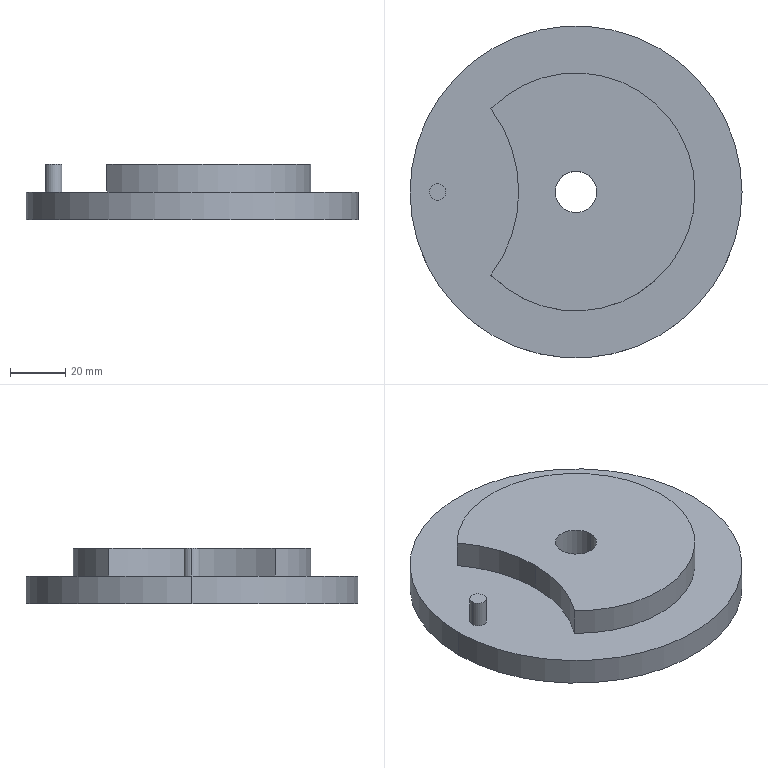Part | STEP file | 1 solid | 14 faces | box 120 x 120 x 20 mm | volume 158754 mm3 | cylinder 10 | plane 4 | commonest cylinder face diameters 6 x2 15 x2 86 x2 100 x2 120 x2
STEP:
#1=CARTESIAN_POINT('',(0.,0.,0.));
#2=DIRECTION('',(0.,0.,1.));
#3=DIRECTION('',(1.,0.,0.));
#4=AXIS2_PLACEMENT_3D('',#1,#2,#3);
#5=CARTESIAN_POINT('',(63.211,0.,10.));
#6=VERTEX_POINT('',#5);
#7=CARTESIAN_POINT('',(63.211,0.,-10.));
#8=VERTEX_POINT('',#7);
#9=CARTESIAN_POINT('',(63.211,0.,-83.));
#10=DIRECTION('',(0.,0.,-1.));
#11=VECTOR('',#10,1.);
#12=LINE('',#9,#11);
#13=CARTESIAN_POINT('',(70.711,0.,-83.));
#14=DIRECTION('',(0.,0.,-1.));
#15=DIRECTION('',(-1.,0.,0.));
#16=AXIS2_PLACEMENT_3D('',#13,#14,#15);
#17=CYLINDRICAL_SURFACE('',#16,7.5);
#18=CARTESIAN_POINT('',(6.283,0.));
#19=DIRECTION('',(0.,1.));
#20=VECTOR('',#19,1.);
#21=LINE('',#18,#20);
#22=(GEOMETRIC_REPRESENTATION_CONTEXT(2)PARAMETRIC_REPRESENTATION_CONTEXT()REPRESENTATION_CONTEXT('',''));
#23=DEFINITIONAL_REPRESENTATION('',(#21),#22);
#24=PCURVE('',#17,#23);
#25=CARTESIAN_POINT('',(70.711,0.,-83.));
#26=DIRECTION('',(0.,0.,-1.));
#27=DIRECTION('',(-1.,0.,0.));
#28=AXIS2_PLACEMENT_3D('',#25,#26,#27);
#29=CYLINDRICAL_SURFACE('',#28,7.5);
#30=CARTESIAN_POINT('',(0.,0.));
#31=DIRECTION('',(0.,1.));
#32=VECTOR('',#31,1.);
#33=LINE('',#30,#32);
#34=(GEOMETRIC_REPRESENTATION_CONTEXT(2)PARAMETRIC_REPRESENTATION_CONTEXT()REPRESENTATION_CONTEXT('',''));
#35=DEFINITIONAL_REPRESENTATION('',(#33),#34);
#36=PCURVE('',#29,#35);
#37=SURFACE_CURVE('',#12,(#24,#36),.PCURVE_S1.);
#38=EDGE_CURVE('',#6,#8,#37,.T.);
#39=ORIENTED_EDGE('',*,*,#38,.T.);
#40=CARTESIAN_POINT('',(78.211,0.,-10.));
#41=VERTEX_POINT('',#40);
#42=CARTESIAN_POINT('',(70.711,0.,-10.));
#43=DIRECTION('',(0.,0.,1.));
#44=DIRECTION('',(-1.,0.,0.));
#45=AXIS2_PLACEMENT_3D('',#42,#43,#44);
#46=CIRCLE('',#45,7.5);
#47=CARTESIAN_POINT('',(6.283,-73.));
#48=DIRECTION('',(-1.,0.));
#49=VECTOR('',#48,1.);
#50=LINE('',#47,#49);
#51=(GEOMETRIC_REPRESENTATION_CONTEXT(2)PARAMETRIC_REPRESENTATION_CONTEXT()REPRESENTATION_CONTEXT('',''));
#52=DEFINITIONAL_REPRESENTATION('',(#50),#51);
#53=PCURVE('',#17,#52);
#54=CARTESIAN_POINT('',(70.711,0.,-10.));
#55=DIRECTION('',(0.,0.,-1.));
#56=DIRECTION('',(-1.,0.,0.));
#57=AXIS2_PLACEMENT_3D('',#54,#55,#56);
#58=PLANE('',#57);
#59=CARTESIAN_POINT('',(7.5,0.));
#60=CARTESIAN_POINT('',(7.5,-12.99));
#61=CARTESIAN_POINT('',(-3.75,-6.495));
#62=CARTESIAN_POINT('',(-15.,0.));
#63=CARTESIAN_POINT('',(-3.75,6.495));
#64=CARTESIAN_POINT('',(7.5,12.99));
#65=CARTESIAN_POINT('',(7.5,0.));
#66=(BOUNDED_CURVE()B_SPLINE_CURVE(2,(#59,#60,#61,#62,#63,#64,#65),.UNSPECIFIED.,.T.,.F.)B_SPLINE_CURVE_WITH_KNOTS((1,2,2,2,2,1),(-2.094,0.,2.094,4.189,6.283,8.378),.UNSPECIFIED.)CURVE()GEOMETRIC_REPRESENTATION_ITEM()RATIONAL_B_SPLINE_CURVE((1.,0.5,1.,0.5,1.,0.5,1.))REPRESENTATION_ITEM(''));
#67=(GEOMETRIC_REPRESENTATION_CONTEXT(2)PARAMETRIC_REPRESENTATION_CONTEXT()REPRESENTATION_CONTEXT('',''));
#68=DEFINITIONAL_REPRESENTATION('',(#66),#67);
#69=PCURVE('',#58,#68);
#70=SURFACE_CURVE('',#46,(#53,#69),.PCURVE_S1.);
#71=EDGE_CURVE('',#8,#41,#70,.T.);
#72=ORIENTED_EDGE('',*,*,#71,.T.);
#73=CARTESIAN_POINT('',(78.211,0.,10.));
#74=VERTEX_POINT('',#73);
#75=CARTESIAN_POINT('',(78.211,0.,-83.));
#76=DIRECTION('',(0.,0.,-1.));
#77=VECTOR('',#76,1.);
#78=LINE('',#75,#77);
#79=CARTESIAN_POINT('',(3.142,0.));
#80=DIRECTION('',(0.,1.));
#81=VECTOR('',#80,1.);
#82=LINE('',#79,#81);
#83=(GEOMETRIC_REPRESENTATION_CONTEXT(2)PARAMETRIC_REPRESENTATION_CONTEXT()REPRESENTATION_CONTEXT('',''));
#84=DEFINITIONAL_REPRESENTATION('',(#82),#83);
#85=PCURVE('',#17,#84);
#86=CARTESIAN_POINT('',(3.142,0.));
#87=DIRECTION('',(0.,1.));
#88=VECTOR('',#87,1.);
#89=LINE('',#86,#88);
#90=(GEOMETRIC_REPRESENTATION_CONTEXT(2)PARAMETRIC_REPRESENTATION_CONTEXT()REPRESENTATION_CONTEXT('',''));
#91=DEFINITIONAL_REPRESENTATION('',(#89),#90);
#92=PCURVE('',#29,#91);
#93=SURFACE_CURVE('',#78,(#85,#92),.PCURVE_S1.);
#94=EDGE_CURVE('',#74,#41,#93,.T.);
#95=ORIENTED_EDGE('',*,*,#94,.F.);
#96=CARTESIAN_POINT('',(70.711,0.,10.));
#97=DIRECTION('',(0.,0.,-1.));
#98=DIRECTION('',(-1.,0.,0.));
#99=AXIS2_PLACEMENT_3D('',#96,#97,#98);
#100=CIRCLE('',#99,7.5);
#101=CARTESIAN_POINT('',(0.,-93.));
#102=DIRECTION('',(1.,0.));
#103=VECTOR('',#102,1.);
#104=LINE('',#101,#103);
#105=(GEOMETRIC_REPRESENTATION_CONTEXT(2)PARAMETRIC_REPRESENTATION_CONTEXT()REPRESENTATION_CONTEXT('',''));
#106=DEFINITIONAL_REPRESENTATION('',(#104),#105);
#107=PCURVE('',#17,#106);
#108=CARTESIAN_POINT('',(0.,0.,10.));
#109=DIRECTION('',(0.,0.,1.));
#110=DIRECTION('',(1.,0.,0.));
#111=AXIS2_PLACEMENT_3D('',#108,#109,#110);
#112=PLANE('',#111);
#113=CARTESIAN_POINT('',(63.211,0.));
#114=CARTESIAN_POINT('',(63.211,12.99));
#115=CARTESIAN_POINT('',(74.461,6.495));
#116=CARTESIAN_POINT('',(85.711,0.));
#117=CARTESIAN_POINT('',(74.461,-6.495));
#118=CARTESIAN_POINT('',(63.211,-12.99));
#119=CARTESIAN_POINT('',(63.211,0.));
#120=(BOUNDED_CURVE()B_SPLINE_CURVE(2,(#113,#114,#115,#116,#117,#118,#119),.UNSPECIFIED.,.T.,.F.)B_SPLINE_CURVE_WITH_KNOTS((1,2,2,2,2,1),(-2.094,0.,2.094,4.189,6.283,8.378),.UNSPECIFIED.)CURVE()GEOMETRIC_REPRESENTATION_ITEM()RATIONAL_B_SPLINE_CURVE((1.,0.5,1.,0.5,1.,0.5,1.))REPRESENTATION_ITEM(''));
#121=(GEOMETRIC_REPRESENTATION_CONTEXT(2)PARAMETRIC_REPRESENTATION_CONTEXT()REPRESENTATION_CONTEXT('',''));
#122=DEFINITIONAL_REPRESENTATION('',(#120),#121);
#123=PCURVE('',#112,#122);
#124=SURFACE_CURVE('',#100,(#107,#123),.PCURVE_S1.);
#125=EDGE_CURVE('',#74,#6,#124,.T.);
#126=ORIENTED_EDGE('',*,*,#125,.T.);
#127=EDGE_LOOP('',(#39,#72,#95,#126));
#128=FACE_BOUND('',#127,.F.);
#129=ADVANCED_FACE('',(#128),#17,.F.);
#130=CARTESIAN_POINT('',(10.711,0.,0.));
#131=VERTEX_POINT('',#130);
#132=CARTESIAN_POINT('',(130.711,0.,0.));
#133=VERTEX_POINT('',#132);
#134=CARTESIAN_POINT('',(70.711,0.,0.));
#135=DIRECTION('',(0.,0.,-1.));
#136=DIRECTION('',(-1.,0.,0.));
#137=AXIS2_PLACEMENT_3D('',#134,#135,#136);
#138=CIRCLE('',#137,60.);
#139=CARTESIAN_POINT('',(70.711,0.,-10.));
#140=DIRECTION('',(0.,0.,-1.));
#141=DIRECTION('',(-1.,0.,0.));
#142=AXIS2_PLACEMENT_3D('',#139,#140,#141);
#143=CYLINDRICAL_SURFACE('',#142,60.);
#144=CARTESIAN_POINT('',(0.,-10.));
#145=DIRECTION('',(1.,0.));
#146=VECTOR('',#145,1.);
#147=LINE('',#144,#146);
#148=(GEOMETRIC_REPRESENTATION_CONTEXT(2)PARAMETRIC_REPRESENTATION_CONTEXT()REPRESENTATION_CONTEXT('',''));
#149=DEFINITIONAL_REPRESENTATION('',(#147),#148);
#150=PCURVE('',#143,#149);
#151=CARTESIAN_POINT('',(70.711,0.,0.));
#152=DIRECTION('',(0.,0.,-1.));
#153=DIRECTION('',(-1.,0.,0.));
#154=AXIS2_PLACEMENT_3D('',#151,#152,#153);
#155=PLANE('',#154);
#156=CARTESIAN_POINT('',(0.,0.));
#157=DIRECTION('',(1.,0.));
#158=AXIS2_PLACEMENT_2D('',#156,#157);
#159=CIRCLE('',#158,60.);
#160=(GEOMETRIC_REPRESENTATION_CONTEXT(2)PARAMETRIC_REPRESENTATION_CONTEXT()REPRESENTATION_CONTEXT('',''));
#161=DEFINITIONAL_REPRESENTATION('',(#159),#160);
#162=PCURVE('',#155,#161);
#163=SURFACE_CURVE('',#138,(#150,#162),.PCURVE_S1.);
#164=EDGE_CURVE('',#131,#133,#163,.T.);
#165=ORIENTED_EDGE('',*,*,#164,.T.);
#166=CARTESIAN_POINT('',(130.711,0.,-10.));
#167=VERTEX_POINT('',#166);
#168=CARTESIAN_POINT('',(130.711,0.,-10.));
#169=DIRECTION('',(0.,0.,-1.));
#170=VECTOR('',#169,1.);
#171=LINE('',#168,#170);
#172=CARTESIAN_POINT('',(3.142,0.));
#173=DIRECTION('',(0.,1.));
#174=VECTOR('',#173,1.);
#175=LINE('',#172,#174);
#176=(GEOMETRIC_REPRESENTATION_CONTEXT(2)PARAMETRIC_REPRESENTATION_CONTEXT()REPRESENTATION_CONTEXT('',''));
#177=DEFINITIONAL_REPRESENTATION('',(#175),#176);
#178=PCURVE('',#143,#177);
#179=CARTESIAN_POINT('',(70.711,0.,-10.));
#180=DIRECTION('',(0.,0.,-1.));
#181=DIRECTION('',(-1.,0.,0.));
#182=AXIS2_PLACEMENT_3D('',#179,#180,#181);
#183=CYLINDRICAL_SURFACE('',#182,60.);
#184=CARTESIAN_POINT('',(3.142,0.));
#185=DIRECTION('',(0.,1.));
#186=VECTOR('',#185,1.);
#187=LINE('',#184,#186);
#188=(GEOMETRIC_REPRESENTATION_CONTEXT(2)PARAMETRIC_REPRESENTATION_CONTEXT()REPRESENTATION_CONTEXT('',''));
#189=DEFINITIONAL_REPRESENTATION('',(#187),#188);
#190=PCURVE('',#183,#189);
#191=SURFACE_CURVE('',#171,(#178,#190),.PCURVE_S1.);
#192=EDGE_CURVE('',#133,#167,#191,.T.);
#193=ORIENTED_EDGE('',*,*,#192,.T.);
#194=CARTESIAN_POINT('',(10.711,0.,-10.));
#195=VERTEX_POINT('',#194);
#196=CARTESIAN_POINT('',(70.711,0.,-10.));
#197=DIRECTION('',(0.,0.,-1.));
#198=DIRECTION('',(-1.,0.,0.));
#199=AXIS2_PLACEMENT_3D('',#196,#197,#198);
#200=CIRCLE('',#199,60.);
#201=CARTESIAN_POINT('',(0.,0.));
#202=DIRECTION('',(1.,0.));
#203=VECTOR('',#202,1.);
#204=LINE('',#201,#203);
#205=(GEOMETRIC_REPRESENTATION_CONTEXT(2)PARAMETRIC_REPRESENTATION_CONTEXT()REPRESENTATION_CONTEXT('',''));
#206=DEFINITIONAL_REPRESENTATION('',(#204),#205);
#207=PCURVE('',#143,#206);
#208=CARTESIAN_POINT('',(0.,0.));
#209=DIRECTION('',(1.,0.));
#210=AXIS2_PLACEMENT_2D('',#208,#209);
#211=CIRCLE('',#210,60.);
#212=(GEOMETRIC_REPRESENTATION_CONTEXT(2)PARAMETRIC_REPRESENTATION_CONTEXT()REPRESENTATION_CONTEXT('',''));
#213=DEFINITIONAL_REPRESENTATION('',(#211),#212);
#214=PCURVE('',#58,#213);
#215=SURFACE_CURVE('',#200,(#207,#214),.PCURVE_S1.);
#216=EDGE_CURVE('',#195,#167,#215,.T.);
#217=ORIENTED_EDGE('',*,*,#216,.F.);
#218=CARTESIAN_POINT('',(10.711,0.,-10.));
#219=DIRECTION('',(0.,0.,-1.));
#220=VECTOR('',#219,1.);
#221=LINE('',#218,#220);
#222=CARTESIAN_POINT('',(0.,0.));
#223=DIRECTION('',(0.,1.));
#224=VECTOR('',#223,1.);
#225=LINE('',#222,#224);
#226=(GEOMETRIC_REPRESENTATION_CONTEXT(2)PARAMETRIC_REPRESENTATION_CONTEXT()REPRESENTATION_CONTEXT('',''));
#227=DEFINITIONAL_REPRESENTATION('',(#225),#226);
#228=PCURVE('',#143,#227);
#229=CARTESIAN_POINT('',(6.283,0.));
#230=DIRECTION('',(0.,1.));
#231=VECTOR('',#230,1.);
#232=LINE('',#229,#231);
#233=(GEOMETRIC_REPRESENTATION_CONTEXT(2)PARAMETRIC_REPRESENTATION_CONTEXT()REPRESENTATION_CONTEXT('',''));
#234=DEFINITIONAL_REPRESENTATION('',(#232),#233);
#235=PCURVE('',#183,#234);
#236=SURFACE_CURVE('',#221,(#228,#235),.PCURVE_S1.);
#237=EDGE_CURVE('',#131,#195,#236,.T.);
#238=ORIENTED_EDGE('',*,*,#237,.F.);
#239=EDGE_LOOP('',(#165,#193,#217,#238));
#240=FACE_BOUND('',#239,.T.);
#241=ADVANCED_FACE('',(#240),#143,.T.);
#242=CARTESIAN_POINT('',(39.959,30.055,0.));
#243=VERTEX_POINT('',#242);
#244=CARTESIAN_POINT('',(39.959,30.055,10.));
#245=VERTEX_POINT('',#244);
#246=CARTESIAN_POINT('',(39.959,30.055,10.));
#247=DIRECTION('',(0.,0.,1.));
#248=VECTOR('',#247,1.);
#249=LINE('',#246,#248);
#250=CARTESIAN_POINT('',(0.,0.,10.));
#251=DIRECTION('',(0.,0.,1.));
#252=DIRECTION('',(1.,0.,0.));
#253=AXIS2_PLACEMENT_3D('',#250,#251,#252);
#254=CYLINDRICAL_SURFACE('',#253,50.);
#255=CARTESIAN_POINT('',(0.6449,0.));
#256=DIRECTION('',(0.,1.));
#257=VECTOR('',#256,1.);
#258=LINE('',#255,#257);
#259=(GEOMETRIC_REPRESENTATION_CONTEXT(2)PARAMETRIC_REPRESENTATION_CONTEXT()REPRESENTATION_CONTEXT('',''));
#260=DEFINITIONAL_REPRESENTATION('',(#258),#259);
#261=PCURVE('',#254,#260);
#262=CARTESIAN_POINT('',(70.711,0.,10.));
#263=DIRECTION('',(0.,0.,1.));
#264=DIRECTION('',(1.,0.,0.));
#265=AXIS2_PLACEMENT_3D('',#262,#263,#264);
#266=CYLINDRICAL_SURFACE('',#265,43.);
#267=CARTESIAN_POINT('',(2.368,0.));
#268=DIRECTION('',(0.,1.));
#269=VECTOR('',#268,1.);
#270=LINE('',#267,#269);
#271=(GEOMETRIC_REPRESENTATION_CONTEXT(2)PARAMETRIC_REPRESENTATION_CONTEXT()REPRESENTATION_CONTEXT('',''));
#272=DEFINITIONAL_REPRESENTATION('',(#270),#271);
#273=PCURVE('',#266,#272);
#274=SURFACE_CURVE('',#249,(#261,#273),.PCURVE_S1.);
#275=EDGE_CURVE('',#243,#245,#274,.T.);
#276=ORIENTED_EDGE('',*,*,#275,.T.);
#277=CARTESIAN_POINT('',(50.,0.,10.));
#278=VERTEX_POINT('',#277);
#279=CARTESIAN_POINT('',(0.,0.,10.));
#280=DIRECTION('',(0.,0.,-1.));
#281=DIRECTION('',(1.,0.,0.));
#282=AXIS2_PLACEMENT_3D('',#279,#280,#281);
#283=CIRCLE('',#282,50.);
#284=CARTESIAN_POINT('',(6.283,0.));
#285=DIRECTION('',(-1.,0.));
#286=VECTOR('',#285,1.);
#287=LINE('',#284,#286);
#288=(GEOMETRIC_REPRESENTATION_CONTEXT(2)PARAMETRIC_REPRESENTATION_CONTEXT()REPRESENTATION_CONTEXT('',''));
#289=DEFINITIONAL_REPRESENTATION('',(#287),#288);
#290=PCURVE('',#254,#289);
#291=CARTESIAN_POINT('',(50.,0.));
#292=CARTESIAN_POINT('',(50.,-86.603));
#293=CARTESIAN_POINT('',(-25.,-43.301));
#294=CARTESIAN_POINT('',(-100.,0.));
#295=CARTESIAN_POINT('',(-25.,43.301));
#296=CARTESIAN_POINT('',(50.,86.603));
#297=CARTESIAN_POINT('',(50.,0.));
#298=(BOUNDED_CURVE()B_SPLINE_CURVE(2,(#291,#292,#293,#294,#295,#296,#297),.UNSPECIFIED.,.T.,.F.)B_SPLINE_CURVE_WITH_KNOTS((1,2,2,2,2,1),(-2.094,0.,2.094,4.189,6.283,8.378),.UNSPECIFIED.)CURVE()GEOMETRIC_REPRESENTATION_ITEM()RATIONAL_B_SPLINE_CURVE((1.,0.5,1.,0.5,1.,0.5,1.))REPRESENTATION_ITEM(''));
#299=(GEOMETRIC_REPRESENTATION_CONTEXT(2)PARAMETRIC_REPRESENTATION_CONTEXT()REPRESENTATION_CONTEXT('',''));
#300=DEFINITIONAL_REPRESENTATION('',(#298),#299);
#301=PCURVE('',#112,#300);
#302=SURFACE_CURVE('',#283,(#290,#301),.PCURVE_S1.);
#303=EDGE_CURVE('',#245,#278,#302,.T.);
#304=ORIENTED_EDGE('',*,*,#303,.T.);
#305=CARTESIAN_POINT('',(50.,0.,0.));
#306=VERTEX_POINT('',#305);
#307=CARTESIAN_POINT('',(50.,0.,10.));
#308=DIRECTION('',(0.,0.,1.));
#309=VECTOR('',#308,1.);
#310=LINE('',#307,#309);
#311=CARTESIAN_POINT('',(0.,0.));
#312=DIRECTION('',(0.,1.));
#313=VECTOR('',#312,1.);
#314=LINE('',#311,#313);
#315=(GEOMETRIC_REPRESENTATION_CONTEXT(2)PARAMETRIC_REPRESENTATION_CONTEXT()REPRESENTATION_CONTEXT('',''));
#316=DEFINITIONAL_REPRESENTATION('',(#314),#315);
#317=PCURVE('',#254,#316);
#318=CARTESIAN_POINT('',(0.,0.,10.));
#319=DIRECTION('',(0.,0.,1.));
#320=DIRECTION('',(1.,0.,0.));
#321=AXIS2_PLACEMENT_3D('',#318,#319,#320);
#322=CYLINDRICAL_SURFACE('',#321,50.);
#323=CARTESIAN_POINT('',(6.283,0.));
#324=DIRECTION('',(0.,1.));
#325=VECTOR('',#324,1.);
#326=LINE('',#323,#325);
#327=(GEOMETRIC_REPRESENTATION_CONTEXT(2)PARAMETRIC_REPRESENTATION_CONTEXT()REPRESENTATION_CONTEXT('',''));
#328=DEFINITIONAL_REPRESENTATION('',(#326),#327);
#329=PCURVE('',#322,#328);
#330=SURFACE_CURVE('',#310,(#317,#329),.PCURVE_S1.);
#331=EDGE_CURVE('',#306,#278,#330,.T.);
#332=ORIENTED_EDGE('',*,*,#331,.F.);
#333=CARTESIAN_POINT('',(0.,0.,0.));
#334=DIRECTION('',(0.,0.,-1.));
#335=DIRECTION('',(1.,0.,0.));
#336=AXIS2_PLACEMENT_3D('',#333,#334,#335);
#337=CIRCLE('',#336,50.);
#338=CARTESIAN_POINT('',(6.283,-10.));
#339=DIRECTION('',(-1.,0.));
#340=VECTOR('',#339,1.);
#341=LINE('',#338,#340);
#342=(GEOMETRIC_REPRESENTATION_CONTEXT(2)PARAMETRIC_REPRESENTATION_CONTEXT()REPRESENTATION_CONTEXT('',''));
#343=DEFINITIONAL_REPRESENTATION('',(#341),#342);
#344=PCURVE('',#254,#343);
#345=CARTESIAN_POINT('',(70.711,0.));
#346=DIRECTION('',(-1.,0.));
#347=AXIS2_PLACEMENT_2D('',#345,#346);
#348=CIRCLE('',#347,50.);
#349=(GEOMETRIC_REPRESENTATION_CONTEXT(2)PARAMETRIC_REPRESENTATION_CONTEXT()REPRESENTATION_CONTEXT('',''));
#350=DEFINITIONAL_REPRESENTATION('',(#348),#349);
#351=PCURVE('',#155,#350);
#352=SURFACE_CURVE('',#337,(#344,#351),.PCURVE_S1.);
#353=EDGE_CURVE('',#243,#306,#352,.T.);
#354=ORIENTED_EDGE('',*,*,#353,.F.);
#355=EDGE_LOOP('',(#276,#304,#332,#354));
#356=FACE_BOUND('',#355,.F.);
#357=ADVANCED_FACE('',(#356),#254,.F.);
#358=CARTESIAN_POINT('',(39.959,-30.055,0.));
#359=VERTEX_POINT('',#358);
#360=CARTESIAN_POINT('',(113.711,0.,0.));
#361=VERTEX_POINT('',#360);
#362=CARTESIAN_POINT('',(70.711,0.,0.));
#363=DIRECTION('',(0.,0.,1.));
#364=DIRECTION('',(1.,0.,0.));
#365=AXIS2_PLACEMENT_3D('',#362,#363,#364);
#366=CIRCLE('',#365,43.);
#367=CARTESIAN_POINT('',(70.711,0.,10.));
#368=DIRECTION('',(0.,0.,1.));
#369=DIRECTION('',(1.,0.,0.));
#370=AXIS2_PLACEMENT_3D('',#367,#368,#369);
#371=CYLINDRICAL_SURFACE('',#370,43.);
#372=CARTESIAN_POINT('',(0.,-10.));
#373=DIRECTION('',(1.,0.));
#374=VECTOR('',#373,1.);
#375=LINE('',#372,#374);
#376=(GEOMETRIC_REPRESENTATION_CONTEXT(2)PARAMETRIC_REPRESENTATION_CONTEXT()REPRESENTATION_CONTEXT('',''));
#377=DEFINITIONAL_REPRESENTATION('',(#375),#376);
#378=PCURVE('',#371,#377);
#379=CARTESIAN_POINT('',(-43.,0.));
#380=CARTESIAN_POINT('',(-43.,74.478));
#381=CARTESIAN_POINT('',(21.5,37.239));
#382=CARTESIAN_POINT('',(86.,0.));
#383=CARTESIAN_POINT('',(21.5,-37.239));
#384=CARTESIAN_POINT('',(-43.,-74.478));
#385=CARTESIAN_POINT('',(-43.,0.));
#386=(BOUNDED_CURVE()B_SPLINE_CURVE(2,(#379,#380,#381,#382,#383,#384,#385),.UNSPECIFIED.,.T.,.F.)B_SPLINE_CURVE_WITH_KNOTS((1,2,2,2,2,1),(-2.094,0.,2.094,4.189,6.283,8.378),.UNSPECIFIED.)CURVE()GEOMETRIC_REPRESENTATION_ITEM()RATIONAL_B_SPLINE_CURVE((1.,0.5,1.,0.5,1.,0.5,1.))REPRESENTATION_ITEM(''));
#387=(GEOMETRIC_REPRESENTATION_CONTEXT(2)PARAMETRIC_REPRESENTATION_CONTEXT()REPRESENTATION_CONTEXT('',''));
#388=DEFINITIONAL_REPRESENTATION('',(#386),#387);
#389=PCURVE('',#155,#388);
#390=SURFACE_CURVE('',#366,(#378,#389),.PCURVE_S1.);
#391=EDGE_CURVE('',#359,#361,#390,.T.);
#392=ORIENTED_EDGE('',*,*,#391,.T.);
#393=CARTESIAN_POINT('',(113.711,0.,10.));
#394=VERTEX_POINT('',#393);
#395=CARTESIAN_POINT('',(113.711,0.,10.));
#396=DIRECTION('',(0.,0.,1.));
#397=VECTOR('',#396,1.);
#398=LINE('',#395,#397);
#399=CARTESIAN_POINT('',(6.283,0.));
#400=DIRECTION('',(0.,1.));
#401=VECTOR('',#400,1.);
#402=LINE('',#399,#401);
#403=(GEOMETRIC_REPRESENTATION_CONTEXT(2)PARAMETRIC_REPRESENTATION_CONTEXT()REPRESENTATION_CONTEXT('',''));
#404=DEFINITIONAL_REPRESENTATION('',(#402),#403);
#405=PCURVE('',#371,#404);
#406=CARTESIAN_POINT('',(0.,0.));
#407=DIRECTION('',(0.,1.));
#408=VECTOR('',#407,1.);
#409=LINE('',#406,#408);
#410=(GEOMETRIC_REPRESENTATION_CONTEXT(2)PARAMETRIC_REPRESENTATION_CONTEXT()REPRESENTATION_CONTEXT('',''));
#411=DEFINITIONAL_REPRESENTATION('',(#409),#410);
#412=PCURVE('',#266,#411);
#413=SURFACE_CURVE('',#398,(#405,#412),.PCURVE_S1.);
#414=EDGE_CURVE('',#361,#394,#413,.T.);
#415=ORIENTED_EDGE('',*,*,#414,.T.);
#416=CARTESIAN_POINT('',(39.959,-30.055,10.));
#417=VERTEX_POINT('',#416);
#418=CARTESIAN_POINT('',(70.711,0.,10.));
#419=DIRECTION('',(0.,0.,1.));
#420=DIRECTION('',(1.,0.,0.));
#421=AXIS2_PLACEMENT_3D('',#418,#419,#420);
#422=CIRCLE('',#421,43.);
#423=CARTESIAN_POINT('',(0.,0.));
#424=DIRECTION('',(1.,0.));
#425=VECTOR('',#424,1.);
#426=LINE('',#423,#425);
#427=(GEOMETRIC_REPRESENTATION_CONTEXT(2)PARAMETRIC_REPRESENTATION_CONTEXT()REPRESENTATION_CONTEXT('',''));
#428=DEFINITIONAL_REPRESENTATION('',(#426),#427);
#429=PCURVE('',#371,#428);
#430=CARTESIAN_POINT('',(70.711,0.));
#431=DIRECTION('',(1.,0.));
#432=AXIS2_PLACEMENT_2D('',#430,#431);
#433=CIRCLE('',#432,43.);
#434=(GEOMETRIC_REPRESENTATION_CONTEXT(2)PARAMETRIC_REPRESENTATION_CONTEXT()REPRESENTATION_CONTEXT('',''));
#435=DEFINITIONAL_REPRESENTATION('',(#433),#434);
#436=PCURVE('',#112,#435);
#437=SURFACE_CURVE('',#422,(#429,#436),.PCURVE_S1.);
#438=EDGE_CURVE('',#417,#394,#437,.T.);
#439=ORIENTED_EDGE('',*,*,#438,.F.);
#440=CARTESIAN_POINT('',(39.959,-30.055,10.));
#441=DIRECTION('',(0.,0.,-1.));
#442=VECTOR('',#441,1.);
#443=LINE('',#440,#442);
#444=CARTESIAN_POINT('',(3.916,0.));
#445=DIRECTION('',(0.,-1.));
#446=VECTOR('',#445,1.);
#447=LINE('',#444,#446);
#448=(GEOMETRIC_REPRESENTATION_CONTEXT(2)PARAMETRIC_REPRESENTATION_CONTEXT()REPRESENTATION_CONTEXT('',''));
#449=DEFINITIONAL_REPRESENTATION('',(#447),#448);
#450=PCURVE('',#371,#449);
#451=CARTESIAN_POINT('',(5.638,0.));
#452=DIRECTION('',(0.,-1.));
#453=VECTOR('',#452,1.);
#454=LINE('',#451,#453);
#455=(GEOMETRIC_REPRESENTATION_CONTEXT(2)PARAMETRIC_REPRESENTATION_CONTEXT()REPRESENTATION_CONTEXT('',''));
#456=DEFINITIONAL_REPRESENTATION('',(#454),#455);
#457=PCURVE('',#322,#456);
#458=SURFACE_CURVE('',#443,(#450,#457),.PCURVE_S1.);
#459=EDGE_CURVE('',#417,#359,#458,.T.);
#460=ORIENTED_EDGE('',*,*,#459,.T.);
#461=EDGE_LOOP('',(#392,#415,#439,#460));
#462=FACE_BOUND('',#461,.T.);
#463=ADVANCED_FACE('',(#462),#371,.T.);
#464=CARTESIAN_POINT('',(23.711,0.,0.));
#465=VERTEX_POINT('',#464);
#466=CARTESIAN_POINT('',(17.711,0.,0.));
#467=VERTEX_POINT('',#466);
#468=CARTESIAN_POINT('',(20.711,0.,0.));
#469=DIRECTION('',(0.,0.,1.));
#470=DIRECTION('',(1.,0.,0.));
#471=AXIS2_PLACEMENT_3D('',#468,#469,#470);
#472=CIRCLE('',#471,3.);
#473=CARTESIAN_POINT('',(20.711,0.,10.));
#474=DIRECTION('',(0.,0.,1.));
#475=DIRECTION('',(1.,0.,0.));
#476=AXIS2_PLACEMENT_3D('',#473,#474,#475);
#477=CYLINDRICAL_SURFACE('',#476,3.);
#478=CARTESIAN_POINT('',(0.,-10.));
#479=DIRECTION('',(1.,0.));
#480=VECTOR('',#479,1.);
#481=LINE('',#478,#480);
#482=(GEOMETRIC_REPRESENTATION_CONTEXT(2)PARAMETRIC_REPRESENTATION_CONTEXT()REPRESENTATION_CONTEXT('',''));
#483=DEFINITIONAL_REPRESENTATION('',(#481),#482);
#484=PCURVE('',#477,#483);
#485=CARTESIAN_POINT('',(47.,0.));
#486=CARTESIAN_POINT('',(47.,5.196));
#487=CARTESIAN_POINT('',(51.5,2.598));
#488=CARTESIAN_POINT('',(56.,0.));
#489=CARTESIAN_POINT('',(51.5,-2.598));
#490=CARTESIAN_POINT('',(47.,-5.196));
#491=CARTESIAN_POINT('',(47.,0.));
#492=(BOUNDED_CURVE()B_SPLINE_CURVE(2,(#485,#486,#487,#488,#489,#490,#491),.UNSPECIFIED.,.T.,.F.)B_SPLINE_CURVE_WITH_KNOTS((1,2,2,2,2,1),(-2.094,0.,2.094,4.189,6.283,8.378),.UNSPECIFIED.)CURVE()GEOMETRIC_REPRESENTATION_ITEM()RATIONAL_B_SPLINE_CURVE((1.,0.5,1.,0.5,1.,0.5,1.))REPRESENTATION_ITEM(''));
#493=(GEOMETRIC_REPRESENTATION_CONTEXT(2)PARAMETRIC_REPRESENTATION_CONTEXT()REPRESENTATION_CONTEXT('',''));
#494=DEFINITIONAL_REPRESENTATION('',(#492),#493);
#495=PCURVE('',#155,#494);
#496=SURFACE_CURVE('',#472,(#484,#495),.PCURVE_S1.);
#497=EDGE_CURVE('',#465,#467,#496,.T.);
#498=ORIENTED_EDGE('',*,*,#497,.T.);
#499=CARTESIAN_POINT('',(17.711,0.,10.));
#500=VERTEX_POINT('',#499);
#501=CARTESIAN_POINT('',(17.711,0.,10.));
#502=DIRECTION('',(0.,0.,1.));
#503=VECTOR('',#502,1.);
#504=LINE('',#501,#503);
#505=CARTESIAN_POINT('',(3.142,0.));
#506=DIRECTION('',(0.,1.));
#507=VECTOR('',#506,1.);
#508=LINE('',#505,#507);
#509=(GEOMETRIC_REPRESENTATION_CONTEXT(2)PARAMETRIC_REPRESENTATION_CONTEXT()REPRESENTATION_CONTEXT('',''));
#510=DEFINITIONAL_REPRESENTATION('',(#508),#509);
#511=PCURVE('',#477,#510);
#512=CARTESIAN_POINT('',(20.711,0.,10.));
#513=DIRECTION('',(0.,0.,1.));
#514=DIRECTION('',(1.,0.,0.));
#515=AXIS2_PLACEMENT_3D('',#512,#513,#514);
#516=CYLINDRICAL_SURFACE('',#515,3.);
#517=CARTESIAN_POINT('',(3.142,0.));
#518=DIRECTION('',(0.,1.));
#519=VECTOR('',#518,1.);
#520=LINE('',#517,#519);
#521=(GEOMETRIC_REPRESENTATION_CONTEXT(2)PARAMETRIC_REPRESENTATION_CONTEXT()REPRESENTATION_CONTEXT('',''));
#522=DEFINITIONAL_REPRESENTATION('',(#520),#521);
#523=PCURVE('',#516,#522);
#524=SURFACE_CURVE('',#504,(#511,#523),.PCURVE_S1.);
#525=EDGE_CURVE('',#467,#500,#524,.T.);
#526=ORIENTED_EDGE('',*,*,#525,.T.);
#527=CARTESIAN_POINT('',(23.711,0.,10.));
#528=VERTEX_POINT('',#527);
#529=CARTESIAN_POINT('',(20.711,0.,10.));
#530=DIRECTION('',(0.,0.,-1.));
#531=DIRECTION('',(1.,0.,0.));
#532=AXIS2_PLACEMENT_3D('',#529,#530,#531);
#533=CIRCLE('',#532,3.);
#534=CARTESIAN_POINT('',(6.283,0.));
#535=DIRECTION('',(-1.,0.));
#536=VECTOR('',#535,1.);
#537=LINE('',#534,#536);
#538=(GEOMETRIC_REPRESENTATION_CONTEXT(2)PARAMETRIC_REPRESENTATION_CONTEXT()REPRESENTATION_CONTEXT('',''));
#539=DEFINITIONAL_REPRESENTATION('',(#537),#538);
#540=PCURVE('',#477,#539);
#541=CARTESIAN_POINT('',(20.711,0.,10.));
#542=DIRECTION('',(0.,0.,1.));
#543=DIRECTION('',(1.,0.,0.));
#544=AXIS2_PLACEMENT_3D('',#541,#542,#543);
#545=PLANE('',#544);
#546=CARTESIAN_POINT('',(3.,0.));
#547=CARTESIAN_POINT('',(3.,-5.196));
#548=CARTESIAN_POINT('',(-1.5,-2.598));
#549=CARTESIAN_POINT('',(-6.,0.));
#550=CARTESIAN_POINT('',(-1.5,2.598));
#551=CARTESIAN_POINT('',(3.,5.196));
#552=CARTESIAN_POINT('',(3.,0.));
#553=(BOUNDED_CURVE()B_SPLINE_CURVE(2,(#546,#547,#548,#549,#550,#551,#552),.UNSPECIFIED.,.T.,.F.)B_SPLINE_CURVE_WITH_KNOTS((1,2,2,2,2,1),(-2.094,0.,2.094,4.189,6.283,8.378),.UNSPECIFIED.)CURVE()GEOMETRIC_REPRESENTATION_ITEM()RATIONAL_B_SPLINE_CURVE((1.,0.5,1.,0.5,1.,0.5,1.))REPRESENTATION_ITEM(''));
#554=(GEOMETRIC_REPRESENTATION_CONTEXT(2)PARAMETRIC_REPRESENTATION_CONTEXT()REPRESENTATION_CONTEXT('',''));
#555=DEFINITIONAL_REPRESENTATION('',(#553),#554);
#556=PCURVE('',#545,#555);
#557=SURFACE_CURVE('',#533,(#540,#556),.PCURVE_S1.);
#558=EDGE_CURVE('',#500,#528,#557,.T.);
#559=ORIENTED_EDGE('',*,*,#558,.T.);
#560=CARTESIAN_POINT('',(23.711,0.,10.));
#561=DIRECTION('',(0.,0.,1.));
#562=VECTOR('',#561,1.);
#563=LINE('',#560,#562);
#564=CARTESIAN_POINT('',(0.,0.));
#565=DIRECTION('',(0.,1.));
#566=VECTOR('',#565,1.);
#567=LINE('',#564,#566);
#568=(GEOMETRIC_REPRESENTATION_CONTEXT(2)PARAMETRIC_REPRESENTATION_CONTEXT()REPRESENTATION_CONTEXT('',''));
#569=DEFINITIONAL_REPRESENTATION('',(#567),#568);
#570=PCURVE('',#477,#569);
#571=CARTESIAN_POINT('',(6.283,0.));
#572=DIRECTION('',(0.,1.));
#573=VECTOR('',#572,1.);
#574=LINE('',#571,#573);
#575=(GEOMETRIC_REPRESENTATION_CONTEXT(2)PARAMETRIC_REPRESENTATION_CONTEXT()REPRESENTATION_CONTEXT('',''));
#576=DEFINITIONAL_REPRESENTATION('',(#574),#575);
#577=PCURVE('',#516,#576);
#578=SURFACE_CURVE('',#563,(#570,#577),.PCURVE_S1.);
#579=EDGE_CURVE('',#465,#528,#578,.T.);
#580=ORIENTED_EDGE('',*,*,#579,.F.);
#581=EDGE_LOOP('',(#498,#526,#559,#580));
#582=FACE_BOUND('',#581,.T.);
#583=ADVANCED_FACE('',(#582),#477,.T.);
#584=ORIENTED_EDGE('',*,*,#71,.T.);
#585=CARTESIAN_POINT('',(70.711,0.,-10.));
#586=DIRECTION('',(0.,0.,1.));
#587=DIRECTION('',(-1.,0.,0.));
#588=AXIS2_PLACEMENT_3D('',#585,#586,#587);
#589=CIRCLE('',#588,7.5);
#590=CARTESIAN_POINT('',(7.5,0.));
#591=CARTESIAN_POINT('',(7.5,-12.99));
#592=CARTESIAN_POINT('',(-3.75,-6.495));
#593=CARTESIAN_POINT('',(-15.,0.));
#594=CARTESIAN_POINT('',(-3.75,6.495));
#595=CARTESIAN_POINT('',(7.5,12.99));
#596=CARTESIAN_POINT('',(7.5,0.));
#597=(BOUNDED_CURVE()B_SPLINE_CURVE(2,(#590,#591,#592,#593,#594,#595,#596),.UNSPECIFIED.,.T.,.F.)B_SPLINE_CURVE_WITH_KNOTS((1,2,2,2,2,1),(-2.094,0.,2.094,4.189,6.283,8.378),.UNSPECIFIED.)CURVE()GEOMETRIC_REPRESENTATION_ITEM()RATIONAL_B_SPLINE_CURVE((1.,0.5,1.,0.5,1.,0.5,1.))REPRESENTATION_ITEM(''));
#598=(GEOMETRIC_REPRESENTATION_CONTEXT(2)PARAMETRIC_REPRESENTATION_CONTEXT()REPRESENTATION_CONTEXT('',''));
#599=DEFINITIONAL_REPRESENTATION('',(#597),#598);
#600=PCURVE('',#58,#599);
#601=CARTESIAN_POINT('',(6.283,-73.));
#602=DIRECTION('',(-1.,0.));
#603=VECTOR('',#602,1.);
#604=LINE('',#601,#603);
#605=(GEOMETRIC_REPRESENTATION_CONTEXT(2)PARAMETRIC_REPRESENTATION_CONTEXT()REPRESENTATION_CONTEXT('',''));
#606=DEFINITIONAL_REPRESENTATION('',(#604),#605);
#607=PCURVE('',#29,#606);
#608=SURFACE_CURVE('',#589,(#600,#607),.PCURVE_S1.);
#609=EDGE_CURVE('',#41,#8,#608,.T.);
#610=ORIENTED_EDGE('',*,*,#609,.T.);
#611=EDGE_LOOP('',(#584,#610));
#612=FACE_BOUND('',#611,.T.);
#613=ORIENTED_EDGE('',*,*,#216,.T.);
#614=CARTESIAN_POINT('',(70.711,0.,-10.));
#615=DIRECTION('',(0.,0.,-1.));
#616=DIRECTION('',(-1.,0.,0.));
#617=AXIS2_PLACEMENT_3D('',#614,#615,#616);
#618=CIRCLE('',#617,60.);
#619=CARTESIAN_POINT('',(0.,0.));
#620=DIRECTION('',(1.,0.));
#621=AXIS2_PLACEMENT_2D('',#619,#620);
#622=CIRCLE('',#621,60.);
#623=(GEOMETRIC_REPRESENTATION_CONTEXT(2)PARAMETRIC_REPRESENTATION_CONTEXT()REPRESENTATION_CONTEXT('',''));
#624=DEFINITIONAL_REPRESENTATION('',(#622),#623);
#625=PCURVE('',#58,#624);
#626=CARTESIAN_POINT('',(0.,0.));
#627=DIRECTION('',(1.,0.));
#628=VECTOR('',#627,1.);
#629=LINE('',#626,#628);
#630=(GEOMETRIC_REPRESENTATION_CONTEXT(2)PARAMETRIC_REPRESENTATION_CONTEXT()REPRESENTATION_CONTEXT('',''));
#631=DEFINITIONAL_REPRESENTATION('',(#629),#630);
#632=PCURVE('',#183,#631);
#633=SURFACE_CURVE('',#618,(#625,#632),.PCURVE_S1.);
#634=EDGE_CURVE('',#167,#195,#633,.T.);
#635=ORIENTED_EDGE('',*,*,#634,.T.);
#636=EDGE_LOOP('',(#613,#635));
#637=FACE_BOUND('',#636,.T.);
#638=ADVANCED_FACE('',(#612,#637),#58,.T.);
#639=ORIENTED_EDGE('',*,*,#609,.T.);
#640=ORIENTED_EDGE('',*,*,#38,.F.);
#641=CARTESIAN_POINT('',(70.711,0.,10.));
#642=DIRECTION('',(0.,0.,-1.));
#643=DIRECTION('',(-1.,0.,0.));
#644=AXIS2_PLACEMENT_3D('',#641,#642,#643);
#645=CIRCLE('',#644,7.5);
#646=CARTESIAN_POINT('',(0.,-93.));
#647=DIRECTION('',(1.,0.));
#648=VECTOR('',#647,1.);
#649=LINE('',#646,#648);
#650=(GEOMETRIC_REPRESENTATION_CONTEXT(2)PARAMETRIC_REPRESENTATION_CONTEXT()REPRESENTATION_CONTEXT('',''));
#651=DEFINITIONAL_REPRESENTATION('',(#649),#650);
#652=PCURVE('',#29,#651);
#653=CARTESIAN_POINT('',(63.211,0.));
#654=CARTESIAN_POINT('',(63.211,12.99));
#655=CARTESIAN_POINT('',(74.461,6.495));
#656=CARTESIAN_POINT('',(85.711,0.));
#657=CARTESIAN_POINT('',(74.461,-6.495));
#658=CARTESIAN_POINT('',(63.211,-12.99));
#659=CARTESIAN_POINT('',(63.211,0.));
#660=(BOUNDED_CURVE()B_SPLINE_CURVE(2,(#653,#654,#655,#656,#657,#658,#659),.UNSPECIFIED.,.T.,.F.)B_SPLINE_CURVE_WITH_KNOTS((1,2,2,2,2,1),(-2.094,0.,2.094,4.189,6.283,8.378),.UNSPECIFIED.)CURVE()GEOMETRIC_REPRESENTATION_ITEM()RATIONAL_B_SPLINE_CURVE((1.,0.5,1.,0.5,1.,0.5,1.))REPRESENTATION_ITEM(''));
#661=(GEOMETRIC_REPRESENTATION_CONTEXT(2)PARAMETRIC_REPRESENTATION_CONTEXT()REPRESENTATION_CONTEXT('',''));
#662=DEFINITIONAL_REPRESENTATION('',(#660),#661);
#663=PCURVE('',#112,#662);
#664=SURFACE_CURVE('',#645,(#652,#663),.PCURVE_S1.);
#665=EDGE_CURVE('',#6,#74,#664,.T.);
#666=ORIENTED_EDGE('',*,*,#665,.T.);
#667=ORIENTED_EDGE('',*,*,#94,.T.);
#668=EDGE_LOOP('',(#639,#640,#666,#667));
#669=FACE_BOUND('',#668,.F.);
#670=ADVANCED_FACE('',(#669),#29,.F.);
#671=ORIENTED_EDGE('',*,*,#192,.F.);
#672=CARTESIAN_POINT('',(70.711,0.,0.));
#673=DIRECTION('',(0.,0.,-1.));
#674=DIRECTION('',(-1.,0.,0.));
#675=AXIS2_PLACEMENT_3D('',#672,#673,#674);
#676=CIRCLE('',#675,60.);
#677=CARTESIAN_POINT('',(0.,-10.));
#678=DIRECTION('',(1.,0.));
#679=VECTOR('',#678,1.);
#680=LINE('',#677,#679);
#681=(GEOMETRIC_REPRESENTATION_CONTEXT(2)PARAMETRIC_REPRESENTATION_CONTEXT()REPRESENTATION_CONTEXT('',''));
#682=DEFINITIONAL_REPRESENTATION('',(#680),#681);
#683=PCURVE('',#183,#682);
#684=CARTESIAN_POINT('',(0.,0.));
#685=DIRECTION('',(1.,0.));
#686=AXIS2_PLACEMENT_2D('',#684,#685);
#687=CIRCLE('',#686,60.);
#688=(GEOMETRIC_REPRESENTATION_CONTEXT(2)PARAMETRIC_REPRESENTATION_CONTEXT()REPRESENTATION_CONTEXT('',''));
#689=DEFINITIONAL_REPRESENTATION('',(#687),#688);
#690=PCURVE('',#155,#689);
#691=SURFACE_CURVE('',#676,(#683,#690),.PCURVE_S1.);
#692=EDGE_CURVE('',#133,#131,#691,.T.);
#693=ORIENTED_EDGE('',*,*,#692,.T.);
#694=ORIENTED_EDGE('',*,*,#237,.T.);
#695=ORIENTED_EDGE('',*,*,#634,.F.);
#696=EDGE_LOOP('',(#671,#693,#694,#695));
#697=FACE_BOUND('',#696,.T.);
#698=ADVANCED_FACE('',(#697),#183,.T.);
#699=ORIENTED_EDGE('',*,*,#665,.T.);
#700=ORIENTED_EDGE('',*,*,#125,.T.);
#701=EDGE_LOOP('',(#699,#700));
#702=FACE_BOUND('',#701,.T.);
#703=ORIENTED_EDGE('',*,*,#438,.T.);
#704=CARTESIAN_POINT('',(70.711,0.,10.));
#705=DIRECTION('',(0.,0.,1.));
#706=DIRECTION('',(1.,0.,0.));
#707=AXIS2_PLACEMENT_3D('',#704,#705,#706);
#708=CIRCLE('',#707,43.);
#709=CARTESIAN_POINT('',(70.711,0.));
#710=DIRECTION('',(1.,0.));
#711=AXIS2_PLACEMENT_2D('',#709,#710);
#712=CIRCLE('',#711,43.);
#713=(GEOMETRIC_REPRESENTATION_CONTEXT(2)PARAMETRIC_REPRESENTATION_CONTEXT()REPRESENTATION_CONTEXT('',''));
#714=DEFINITIONAL_REPRESENTATION('',(#712),#713);
#715=PCURVE('',#112,#714);
#716=CARTESIAN_POINT('',(0.,0.));
#717=DIRECTION('',(1.,0.));
#718=VECTOR('',#717,1.);
#719=LINE('',#716,#718);
#720=(GEOMETRIC_REPRESENTATION_CONTEXT(2)PARAMETRIC_REPRESENTATION_CONTEXT()REPRESENTATION_CONTEXT('',''));
#721=DEFINITIONAL_REPRESENTATION('',(#719),#720);
#722=PCURVE('',#266,#721);
#723=SURFACE_CURVE('',#708,(#715,#722),.PCURVE_S1.);
#724=EDGE_CURVE('',#394,#245,#723,.T.);
#725=ORIENTED_EDGE('',*,*,#724,.T.);
#726=ORIENTED_EDGE('',*,*,#303,.T.);
#727=CARTESIAN_POINT('',(0.,0.,10.));
#728=DIRECTION('',(0.,0.,-1.));
#729=DIRECTION('',(1.,0.,0.));
#730=AXIS2_PLACEMENT_3D('',#727,#728,#729);
#731=CIRCLE('',#730,50.);
#732=CARTESIAN_POINT('',(50.,0.));
#733=CARTESIAN_POINT('',(50.,-86.603));
#734=CARTESIAN_POINT('',(-25.,-43.301));
#735=CARTESIAN_POINT('',(-100.,0.));
#736=CARTESIAN_POINT('',(-25.,43.301));
#737=CARTESIAN_POINT('',(50.,86.603));
#738=CARTESIAN_POINT('',(50.,0.));
#739=(BOUNDED_CURVE()B_SPLINE_CURVE(2,(#732,#733,#734,#735,#736,#737,#738),.UNSPECIFIED.,.T.,.F.)B_SPLINE_CURVE_WITH_KNOTS((1,2,2,2,2,1),(-2.094,0.,2.094,4.189,6.283,8.378),.UNSPECIFIED.)CURVE()GEOMETRIC_REPRESENTATION_ITEM()RATIONAL_B_SPLINE_CURVE((1.,0.5,1.,0.5,1.,0.5,1.))REPRESENTATION_ITEM(''));
#740=(GEOMETRIC_REPRESENTATION_CONTEXT(2)PARAMETRIC_REPRESENTATION_CONTEXT()REPRESENTATION_CONTEXT('',''));
#741=DEFINITIONAL_REPRESENTATION('',(#739),#740);
#742=PCURVE('',#112,#741);
#743=CARTESIAN_POINT('',(6.283,0.));
#744=DIRECTION('',(-1.,0.));
#745=VECTOR('',#744,1.);
#746=LINE('',#743,#745);
#747=(GEOMETRIC_REPRESENTATION_CONTEXT(2)PARAMETRIC_REPRESENTATION_CONTEXT()REPRESENTATION_CONTEXT('',''));
#748=DEFINITIONAL_REPRESENTATION('',(#746),#747);
#749=PCURVE('',#322,#748);
#750=SURFACE_CURVE('',#731,(#742,#749),.PCURVE_S1.);
#751=EDGE_CURVE('',#278,#417,#750,.T.);
#752=ORIENTED_EDGE('',*,*,#751,.T.);
#753=EDGE_LOOP('',(#703,#725,#726,#752));
#754=FACE_BOUND('',#753,.T.);
#755=ADVANCED_FACE('',(#702,#754),#112,.T.);
#756=ORIENTED_EDGE('',*,*,#353,.F.);
#757=CARTESIAN_POINT('',(70.711,0.,0.));
#758=DIRECTION('',(0.,0.,1.));
#759=DIRECTION('',(1.,0.,0.));
#760=AXIS2_PLACEMENT_3D('',#757,#758,#759);
#761=CIRCLE('',#760,43.);
#762=CARTESIAN_POINT('',(-43.,0.));
#763=CARTESIAN_POINT('',(-43.,74.478));
#764=CARTESIAN_POINT('',(21.5,37.239));
#765=CARTESIAN_POINT('',(86.,0.));
#766=CARTESIAN_POINT('',(21.5,-37.239));
#767=CARTESIAN_POINT('',(-43.,-74.478));
#768=CARTESIAN_POINT('',(-43.,0.));
#769=(BOUNDED_CURVE()B_SPLINE_CURVE(2,(#762,#763,#764,#765,#766,#767,#768),.UNSPECIFIED.,.T.,.F.)B_SPLINE_CURVE_WITH_KNOTS((1,2,2,2,2,1),(-2.094,0.,2.094,4.189,6.283,8.378),.UNSPECIFIED.)CURVE()GEOMETRIC_REPRESENTATION_ITEM()RATIONAL_B_SPLINE_CURVE((1.,0.5,1.,0.5,1.,0.5,1.))REPRESENTATION_ITEM(''));
#770=(GEOMETRIC_REPRESENTATION_CONTEXT(2)PARAMETRIC_REPRESENTATION_CONTEXT()REPRESENTATION_CONTEXT('',''));
#771=DEFINITIONAL_REPRESENTATION('',(#769),#770);
#772=PCURVE('',#155,#771);
#773=CARTESIAN_POINT('',(0.,-10.));
#774=DIRECTION('',(1.,0.));
#775=VECTOR('',#774,1.);
#776=LINE('',#773,#775);
#777=(GEOMETRIC_REPRESENTATION_CONTEXT(2)PARAMETRIC_REPRESENTATION_CONTEXT()REPRESENTATION_CONTEXT('',''));
#778=DEFINITIONAL_REPRESENTATION('',(#776),#777);
#779=PCURVE('',#266,#778);
#780=SURFACE_CURVE('',#761,(#772,#779),.PCURVE_S1.);
#781=EDGE_CURVE('',#361,#243,#780,.T.);
#782=ORIENTED_EDGE('',*,*,#781,.F.);
#783=ORIENTED_EDGE('',*,*,#391,.F.);
#784=CARTESIAN_POINT('',(0.,0.,0.));
#785=DIRECTION('',(0.,0.,-1.));
#786=DIRECTION('',(1.,0.,0.));
#787=AXIS2_PLACEMENT_3D('',#784,#785,#786);
#788=CIRCLE('',#787,50.);
#789=CARTESIAN_POINT('',(70.711,0.));
#790=DIRECTION('',(-1.,0.));
#791=AXIS2_PLACEMENT_2D('',#789,#790);
#792=CIRCLE('',#791,50.);
#793=(GEOMETRIC_REPRESENTATION_CONTEXT(2)PARAMETRIC_REPRESENTATION_CONTEXT()REPRESENTATION_CONTEXT('',''));
#794=DEFINITIONAL_REPRESENTATION('',(#792),#793);
#795=PCURVE('',#155,#794);
#796=CARTESIAN_POINT('',(6.283,-10.));
#797=DIRECTION('',(-1.,0.));
#798=VECTOR('',#797,1.);
#799=LINE('',#796,#798);
#800=(GEOMETRIC_REPRESENTATION_CONTEXT(2)PARAMETRIC_REPRESENTATION_CONTEXT()REPRESENTATION_CONTEXT('',''));
#801=DEFINITIONAL_REPRESENTATION('',(#799),#800);
#802=PCURVE('',#322,#801);
#803=SURFACE_CURVE('',#788,(#795,#802),.PCURVE_S1.);
#804=EDGE_CURVE('',#306,#359,#803,.T.);
#805=ORIENTED_EDGE('',*,*,#804,.F.);
#806=EDGE_LOOP('',(#756,#782,#783,#805));
#807=FACE_BOUND('',#806,.T.);
#808=ORIENTED_EDGE('',*,*,#497,.F.);
#809=CARTESIAN_POINT('',(20.711,0.,0.));
#810=DIRECTION('',(0.,0.,1.));
#811=DIRECTION('',(1.,0.,0.));
#812=AXIS2_PLACEMENT_3D('',#809,#810,#811);
#813=CIRCLE('',#812,3.);
#814=CARTESIAN_POINT('',(47.,0.));
#815=CARTESIAN_POINT('',(47.,5.196));
#816=CARTESIAN_POINT('',(51.5,2.598));
#817=CARTESIAN_POINT('',(56.,0.));
#818=CARTESIAN_POINT('',(51.5,-2.598));
#819=CARTESIAN_POINT('',(47.,-5.196));
#820=CARTESIAN_POINT('',(47.,0.));
#821=(BOUNDED_CURVE()B_SPLINE_CURVE(2,(#814,#815,#816,#817,#818,#819,#820),.UNSPECIFIED.,.T.,.F.)B_SPLINE_CURVE_WITH_KNOTS((1,2,2,2,2,1),(-2.094,0.,2.094,4.189,6.283,8.378),.UNSPECIFIED.)CURVE()GEOMETRIC_REPRESENTATION_ITEM()RATIONAL_B_SPLINE_CURVE((1.,0.5,1.,0.5,1.,0.5,1.))REPRESENTATION_ITEM(''));
#822=(GEOMETRIC_REPRESENTATION_CONTEXT(2)PARAMETRIC_REPRESENTATION_CONTEXT()REPRESENTATION_CONTEXT('',''));
#823=DEFINITIONAL_REPRESENTATION('',(#821),#822);
#824=PCURVE('',#155,#823);
#825=CARTESIAN_POINT('',(0.,-10.));
#826=DIRECTION('',(1.,0.));
#827=VECTOR('',#826,1.);
#828=LINE('',#825,#827);
#829=(GEOMETRIC_REPRESENTATION_CONTEXT(2)PARAMETRIC_REPRESENTATION_CONTEXT()REPRESENTATION_CONTEXT('',''));
#830=DEFINITIONAL_REPRESENTATION('',(#828),#829);
#831=PCURVE('',#516,#830);
#832=SURFACE_CURVE('',#813,(#824,#831),.PCURVE_S1.);
#833=EDGE_CURVE('',#467,#465,#832,.T.);
#834=ORIENTED_EDGE('',*,*,#833,.F.);
#835=EDGE_LOOP('',(#808,#834));
#836=FACE_BOUND('',#835,.T.);
#837=ORIENTED_EDGE('',*,*,#164,.F.);
#838=ORIENTED_EDGE('',*,*,#692,.F.);
#839=EDGE_LOOP('',(#837,#838));
#840=FACE_BOUND('',#839,.T.);
#841=ADVANCED_FACE('',(#807,#836,#840),#155,.F.);
#842=ORIENTED_EDGE('',*,*,#751,.T.);
#843=ORIENTED_EDGE('',*,*,#459,.T.);
#844=ORIENTED_EDGE('',*,*,#804,.F.);
#845=ORIENTED_EDGE('',*,*,#331,.T.);
#846=EDGE_LOOP('',(#842,#843,#844,#845));
#847=FACE_BOUND('',#846,.F.);
#848=ADVANCED_FACE('',(#847),#322,.F.);
#849=ORIENTED_EDGE('',*,*,#414,.F.);
#850=ORIENTED_EDGE('',*,*,#781,.T.);
#851=ORIENTED_EDGE('',*,*,#275,.T.);
#852=ORIENTED_EDGE('',*,*,#724,.F.);
#853=EDGE_LOOP('',(#849,#850,#851,#852));
#854=FACE_BOUND('',#853,.T.);
#855=ADVANCED_FACE('',(#854),#266,.T.);
#856=ORIENTED_EDGE('',*,*,#525,.F.);
#857=ORIENTED_EDGE('',*,*,#833,.T.);
#858=ORIENTED_EDGE('',*,*,#579,.T.);
#859=CARTESIAN_POINT('',(20.711,0.,10.));
#860=DIRECTION('',(0.,0.,-1.));
#861=DIRECTION('',(1.,0.,0.));
#862=AXIS2_PLACEMENT_3D('',#859,#860,#861);
#863=CIRCLE('',#862,3.);
#864=CARTESIAN_POINT('',(6.283,0.));
#865=DIRECTION('',(-1.,0.));
#866=VECTOR('',#865,1.);
#867=LINE('',#864,#866);
#868=(GEOMETRIC_REPRESENTATION_CONTEXT(2)PARAMETRIC_REPRESENTATION_CONTEXT()REPRESENTATION_CONTEXT('',''));
#869=DEFINITIONAL_REPRESENTATION('',(#867),#868);
#870=PCURVE('',#516,#869);
#871=CARTESIAN_POINT('',(3.,0.));
#872=CARTESIAN_POINT('',(3.,-5.196));
#873=CARTESIAN_POINT('',(-1.5,-2.598));
#874=CARTESIAN_POINT('',(-6.,0.));
#875=CARTESIAN_POINT('',(-1.5,2.598));
#876=CARTESIAN_POINT('',(3.,5.196));
#877=CARTESIAN_POINT('',(3.,0.));
#878=(BOUNDED_CURVE()B_SPLINE_CURVE(2,(#871,#872,#873,#874,#875,#876,#877),.UNSPECIFIED.,.T.,.F.)B_SPLINE_CURVE_WITH_KNOTS((1,2,2,2,2,1),(-2.094,0.,2.094,4.189,6.283,8.378),.UNSPECIFIED.)CURVE()GEOMETRIC_REPRESENTATION_ITEM()RATIONAL_B_SPLINE_CURVE((1.,0.5,1.,0.5,1.,0.5,1.))REPRESENTATION_ITEM(''));
#879=(GEOMETRIC_REPRESENTATION_CONTEXT(2)PARAMETRIC_REPRESENTATION_CONTEXT()REPRESENTATION_CONTEXT('',''));
#880=DEFINITIONAL_REPRESENTATION('',(#878),#879);
#881=PCURVE('',#545,#880);
#882=SURFACE_CURVE('',#863,(#870,#881),.PCURVE_S1.);
#883=EDGE_CURVE('',#528,#500,#882,.T.);
#884=ORIENTED_EDGE('',*,*,#883,.T.);
#885=EDGE_LOOP('',(#856,#857,#858,#884));
#886=FACE_BOUND('',#885,.T.);
#887=ADVANCED_FACE('',(#886),#516,.T.);
#888=ORIENTED_EDGE('',*,*,#883,.F.);
#889=ORIENTED_EDGE('',*,*,#558,.F.);
#890=EDGE_LOOP('',(#888,#889));
#891=FACE_BOUND('',#890,.T.);
#892=ADVANCED_FACE('',(#891),#545,.T.);
#893=CLOSED_SHELL('',(#129,#241,#357,#463,#583,#638,#670,#698,#755,#841,#848,#855,#887,#892));
#894=MANIFOLD_SOLID_BREP('',#893);
#895=(LENGTH_UNIT()NAMED_UNIT(*)SI_UNIT(.MILLI.,.METRE.));
#896=UNCERTAINTY_MEASURE_WITH_UNIT(LENGTH_MEASURE(0.0000001),#895,'','');
#897=(NAMED_UNIT(*)PLANE_ANGLE_UNIT()SI_UNIT($,.RADIAN.));
#898=(NAMED_UNIT(*)SI_UNIT($,.STERADIAN.)SOLID_ANGLE_UNIT());
#899=(GEOMETRIC_REPRESENTATION_CONTEXT(3)GLOBAL_UNCERTAINTY_ASSIGNED_CONTEXT((#896))GLOBAL_UNIT_ASSIGNED_CONTEXT((#895,#897,#898))REPRESENTATION_CONTEXT('',''));
#900=ADVANCED_BREP_SHAPE_REPRESENTATION('',(#4,#894),#899);